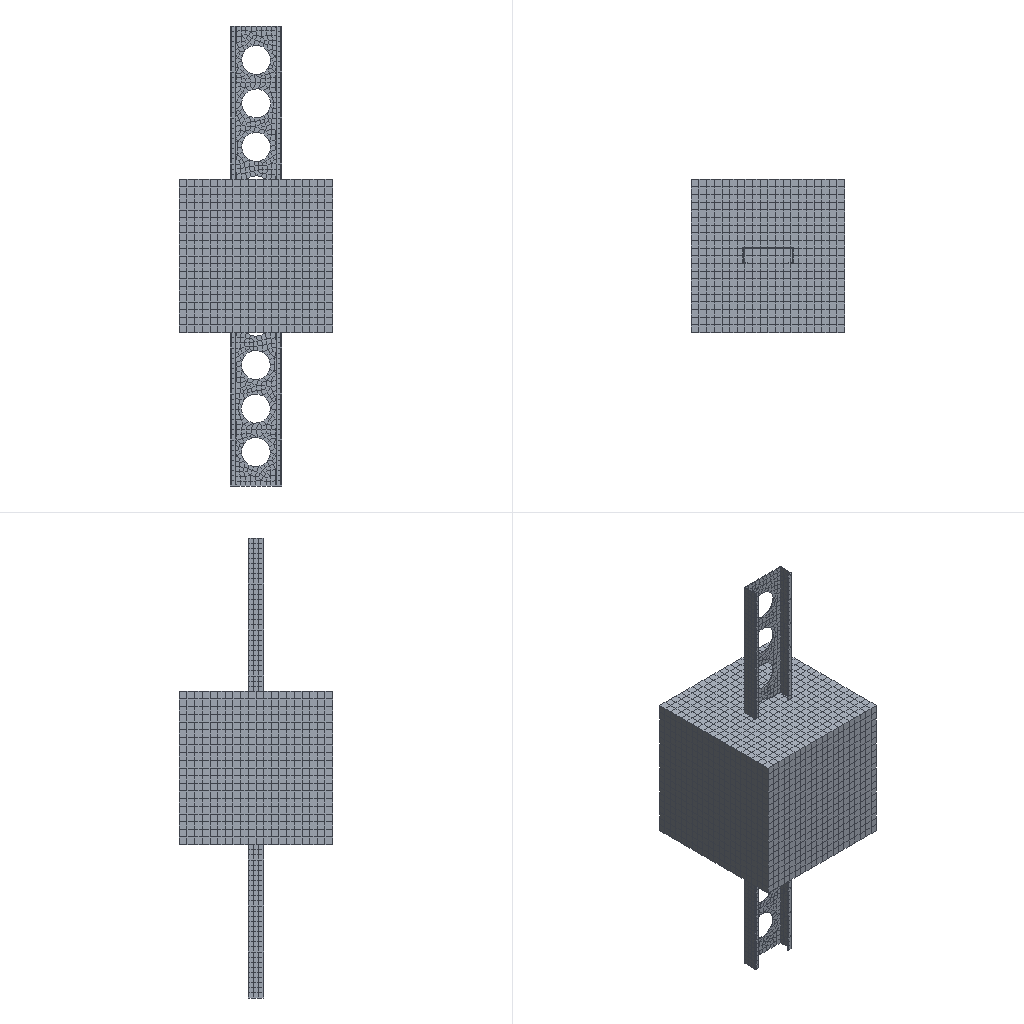Simulation study | abaqus
Set-up summary:
category,name,step,type,value,unit,region
solver,abaqus
solver,version,,,Abaqus/Explicit 2020
units,not stated in the deck,,not stated
analysis,deck,,transient,transient
load_step,Step-1,Step-1,transient
load_step,requested,,,1
mesh,nodes,,,16221
mesh,elements,,,11286
element_type,R3D4,,rigid,192
element_type,C3D8R,,solid,11094
load,load commands in deck,,count,1
bc,support commands in deck,,count,13
material,AL,,in results
material,CON,,in results
material,Q235,,in results
check,setup vs results,,match,"per instance, exact: element labels, types and connectivity; labels of the nodes the elements use; coordinates of those nodes at SINGLE_PRECISION in 7 of 8 instance(s)"
Abaqus input file, long lists of numbers shortened:
*Heading
** Job name: Job-1 Model name: Model-1
** Generated by: Abaqus/CAE 2020
*Preprint, echo=NO, model=NO, history=NO, contact=NO
**
** PARTS
**
*Part, name=Part-1
*Node
      1,        39.75,   29.6,         340.
      2,        39.75,   31.1,         340.
** (2258 more lines like these left out)
*Element, type=C3D8R
 1, 109, 129, 128, 108,   1,   2,   3,   4
 2, 110, 130, 127, 107, 109, 129, 128, 108
** (1014 more lines like these left out)
*Nset, nset=Set-1, generate
    1,  2260,     1
*Elset, elset=Set-1, generate
    1,  1016,     1
** Section: al
*Solid Section, elset=Set-1, material=al
,
*End Part
**
*Part, name=Part-2
*Node
      1,       -27.25,         12.5,         250.
      2,       -27.25,         12.5,           0.
** (2234 more lines like these left out)
*Element, type=C3D8R
 1,   5,  81, 128,   8,   1,  33,  80,   4
 2,  81,  82, 127, 128,  33,  34,  79,  80
** (1060 more lines like these left out)
*Nset, nset=Set-7, generate
    1,  2236,     1
*Elset, elset=Set-7, generate
    1,  1062,     1
** Section: q235
*Solid Section, elset=Set-7, material=q235
,
*End Part
**
*Part, name=Part-3
*Node
      1,          4.5, -0.325,           0.
      2,          4.5,        0.875,           0.
** (48 more lines like these left out)
*Element, type=R3D4
1,  1, 15, 22,  2
2, 15, 14, 21, 22
** (46 more lines like these left out)
*Node
     51,           0.,        0.875,           0.
*Nset, nset=Part-3-RefPt_, internal
51,
*Elset, elset=Part-3, generate
  1,  48,   1
*End Part
**
*Part, name=con
*Node
      1,           0.,        -300.,         300.
      2,           0.,        -285.,         300.
** (9259 more lines like these left out)
*Element, type=C3D8R
   1,  442,  443,  464,  463,    1,    2,   23,   22
   2,  443,  444,  465,  464,    2,    3,   24,   23
** (7998 more lines like these left out)
*Nset, nset=Set-1, generate
    1,  9261,     1
*Elset, elset=Set-1, generate
    1,  8000,     1
** Section: con
*Solid Section, elset=Set-1, material=con
,
*End Part
**
**
** ASSEMBLY
**
*Assembly, name=Assembly
**
*Instance, name=Part-1-1, part=Part-1
*End Instance
**
*Instance, name=Part-1-2, part=Part-1
-17.9,           0.,           0.
-17.9,           0.,           0., -17.9,           1.,           0.,         180.
*End Instance
**
*Instance, name=Part-2-1, part=Part-2
       -31.9,         20.1,        -125.
*End Instance
**
*Instance, name=Part-3-1, part=Part-3
      -34.05,       32.925,        -86.4
*End Instance
**
*Instance, name=Part-3-2, part=Part-3
       16.15,       32.925,        -86.4
*End Instance
**
*Instance, name=Part-3-3, part=Part-3
      -34.05,       32.925,         86.4
*End Instance
**
*Instance, name=Part-3-4, part=Part-3
       16.15,       32.925,         86.4
*End Instance
**
*Instance, name=con-1, part=con
     -158.95,        165.5,        -150.
*End Instance
**
*Node
      1,  -8.95,   15.55,        -450.
*Node
      2,  -8.95,   15.55,         450.
*Nset, nset=Set-5
 1,
*Nset, nset=Set-6
 2,
*Nset, nset=Set-7, instance=Part-3-1
 51,
*Nset, nset=Set-7, instance=Part-3-2
 51,
*Nset, nset=Set-7, instance=Part-3-3
 51,
*Nset, nset=Set-7, instance=Part-3-4
 51,
*Nset, nset=Set-11, instance=Part-2-1
    1,    2,   15,   16,   29,   30,   31,   32,   33,   34,   35,   36,   37,   38,   39,   40
   41,   42,   43,   44,   45,   46,   47,   48,   49,   50,   51,   52,   53,   54,   55,   56
** (55 more lines like these left out)
*Elset, elset=Set-11, instance=Part-2-1, generate
  201,  1062,     1
*Nset, nset=m_Set-1, instance=Part-1-1
   39,   40,   41,   42,   43,   44,   45,   46,   47,   48,   49,   50,   51,   52,   53,   54
   55,   56,   57,   60,   61,   62,   63,   64,   65,   66,   67,   68,   69,   70,   71,   72
** (55 more lines like these left out)
*Nset, nset=m_Set-1, instance=Part-1-2
   39,   40,   41,   42,   43,   44,   45,   46,   47,   48,   49,   50,   51,   52,   53,   54
   55,   56,   57,   60,   61,   62,   63,   64,   65,   66,   67,   68,   69,   70,   71,   72
** (55 more lines like these left out)
*Nset, nset=m_Set-1, instance=Part-3-1, generate
  1,  50,   1
*Nset, nset=m_Set-1, instance=Part-3-3, generate
  1,  50,   1
*Nset, nset=m_Set-1, instance=Part-3-2, generate
  1,  50,   1
*Nset, nset=m_Set-1, instance=Part-3-4, generate
  1,  50,   1
*Elset, elset=m_Set-1, instance=Part-1-1
  361,  362,  363,  364,  365,  366,  367,  368,  369,  370,  371,  372,  373,  374,  375,  376
  377,  378,  379,  380,  381,  382,  383,  384,  385,  386,  387,  388,  389,  390,  391,  392
** (23 more lines like these left out)
*Elset, elset=m_Set-1, instance=Part-1-2
  361,  362,  363,  364,  365,  366,  367,  368,  369,  370,  371,  372,  373,  374,  375,  376
  377,  378,  379,  380,  381,  382,  383,  384,  385,  386,  387,  388,  389,  390,  391,  392
** (23 more lines like these left out)
*Elset, elset=m_Set-1, instance=Part-3-1, generate
  1,  48,   1
*Elset, elset=m_Set-1, instance=Part-3-3, generate
  1,  48,   1
*Elset, elset=m_Set-1, instance=Part-3-2, generate
  1,  48,   1
*Elset, elset=m_Set-1, instance=Part-3-4, generate
  1,  48,   1
*Nset, nset=m_Set-3
 1,
*Nset, nset=m_Set-4
 2,
*Nset, nset=m_Set-9, instance=Part-1-1
   39,   40,   41,   42,   43,   44,   45,   46,   47,   48,   49,   50,   51,   52,   53,   54
   55,   56,   57,   60,   61,   62,   63,   64,   65,   66,   67,   68,   69,   70,   71,   72
** (55 more lines like these left out)
*Nset, nset=m_Set-9, instance=Part-1-2
   39,   40,   41,   42,   43,   44,   45,   46,   47,   48,   49,   50,   51,   52,   53,   54
   55,   56,   57,   60,   61,   62,   63,   64,   65,   66,   67,   68,   69,   70,   71,   72
** (55 more lines like these left out)
*Nset, nset=m_Set-9, instance=Part-3-1, generate
  1,  50,   1
*Nset, nset=m_Set-9, instance=Part-3-3, generate
  1,  50,   1
*Nset, nset=m_Set-9, instance=Part-2-1, generate
    1,  2236,     1
*Nset, nset=m_Set-9, instance=Part-3-2, generate
  1,  50,   1
*Nset, nset=m_Set-9, instance=Part-3-4, generate
  1,  50,   1
*Elset, elset=m_Set-9, instance=Part-1-1
  361,  362,  363,  364,  365,  366,  367,  368,  369,  370,  371,  372,  373,  374,  375,  376
  377,  378,  379,  380,  381,  382,  383,  384,  385,  386,  387,  388,  389,  390,  391,  392
** (23 more lines like these left out)
*Elset, elset=m_Set-9, instance=Part-1-2
  361,  362,  363,  364,  365,  366,  367,  368,  369,  370,  371,  372,  373,  374,  375,  376
  377,  378,  379,  380,  381,  382,  383,  384,  385,  386,  387,  388,  389,  390,  391,  392
** (23 more lines like these left out)
*Elset, elset=m_Set-9, instance=Part-3-1, generate
  1,  48,   1
*Elset, elset=m_Set-9, instance=Part-3-3, generate
  1,  48,   1
*Elset, elset=m_Set-9, instance=Part-2-1, generate
    1,  1062,     1
*Elset, elset=m_Set-9, instance=Part-3-2, generate
  1,  48,   1
*Elset, elset=m_Set-9, instance=Part-3-4, generate
  1,  48,   1
*Nset, nset=s_Set-1, instance=con-1, generate
    1,  9261,     1
*Elset, elset=s_Set-1, instance=con-1, generate
    1,  8000,     1
*Nset, nset=s_Set-9, instance=con-1, generate
    1,  9261,     1
*Elset, elset=s_Set-9, instance=con-1, generate
    1,  8000,     1
*Elset, elset=_m_Surf-3_S5, internal, instance=Part-1-1
  361,  362,  363,  364,  365,  366,  367,  368,  369,  370,  371,  372,  373,  374,  375,  376
  377,  378,  379,  380,  381,  382,  383,  384,  385,  386,  387,  388,  389,  390,  436,  437
** (3 more lines like these left out)
*Elset, elset=_m_Surf-3_S4, internal, instance=Part-1-1
  361,  362,  363,  364,  365,  366,  367,  368,  369,  370,  371,  372,  373,  374,  375,  376
  377,  378,  379,  380,  381,  382,  383,  384,  385,  386,  387,  388,  389,  390,  391,  392
** (9 more lines like these left out)
*Elset, elset=_m_Surf-3_S3, internal, instance=Part-1-1
 466, 467, 468, 469, 470, 471, 472, 473, 474, 475, 476, 477, 478, 479, 480, 814
 851, 878, 920, 981
*Elset, elset=_m_Surf-3_S2, internal, instance=Part-1-1, generate
  802,  1016,     1
*Elset, elset=_m_Surf-3_S6, internal, instance=Part-1-1
 376, 377, 378, 379, 380, 381, 382, 383, 384, 385, 386, 387, 388, 389, 390, 391
 392, 393, 394, 395, 396, 397, 398, 399, 400, 401, 402, 403, 404, 405, 406, 407
** (7 more lines like these left out)
*Elset, elset=_m_Surf-3_S1, internal, instance=Part-1-1, generate
  802,  1016,     1
*Surface, type=ELEMENT, name=m_Surf-3
_m_Surf-3_S5, S5
_m_Surf-3_S4, S4
_m_Surf-3_S2, S2
_m_Surf-3_S6, S6
_m_Surf-3_S3, S3
_m_Surf-3_S1, S1
*Elset, elset=_m_Surf-6_SPOS, internal, instance=Part-3-4, generate
  1,  48,   1
*Surface, type=ELEMENT, name=m_Surf-6
_m_Surf-6_SPOS, SPOS
*Elset, elset=_m_Surf-8_SPOS, internal, instance=Part-3-3, generate
  1,  48,   1
*Surface, type=ELEMENT, name=m_Surf-8
_m_Surf-8_SPOS, SPOS
*Elset, elset=_m_Surf-10_S5, internal, instance=Part-1-2
  361,  362,  363,  364,  365,  366,  367,  368,  369,  370,  371,  372,  373,  374,  375,  376
  377,  378,  379,  380,  381,  382,  383,  384,  385,  386,  387,  388,  389,  390,  436,  437
** (3 more lines like these left out)
*Elset, elset=_m_Surf-10_S4, internal, instance=Part-1-2
  361,  362,  363,  364,  365,  366,  367,  368,  369,  370,  371,  372,  373,  374,  375,  376
  377,  378,  379,  380,  381,  382,  383,  384,  385,  386,  387,  388,  389,  390,  391,  392
** (9 more lines like these left out)
*Elset, elset=_m_Surf-10_S3, internal, instance=Part-1-2
 466, 467, 468, 469, 470, 471, 472, 473, 474, 475, 476, 477, 478, 479, 480, 814
 851, 878, 920, 981
*Elset, elset=_m_Surf-10_S2, internal, instance=Part-1-2, generate
  802,  1016,     1
*Elset, elset=_m_Surf-10_S6, internal, instance=Part-1-2
 376, 377, 378, 379, 380, 381, 382, 383, 384, 385, 386, 387, 388, 389, 390, 391
 392, 393, 394, 395, 396, 397, 398, 399, 400, 401, 402, 403, 404, 405, 406, 407
** (7 more lines like these left out)
*Elset, elset=_m_Surf-10_S1, internal, instance=Part-1-2, generate
  802,  1016,     1
*Surface, type=ELEMENT, name=m_Surf-10
_m_Surf-10_S5, S5
_m_Surf-10_S4, S4
_m_Surf-10_S2, S2
_m_Surf-10_S6, S6
_m_Surf-10_S3, S3
_m_Surf-10_S1, S1
*Elset, elset=_m_Surf-13_SPOS, internal, instance=Part-3-1, generate
  1,  48,   1
*Surface, type=ELEMENT, name=m_Surf-13
_m_Surf-13_SPOS, SPOS
*Elset, elset=_m_Surf-15_SPOS, internal, instance=Part-3-2, generate
  1,  48,   1
*Surface, type=ELEMENT, name=m_Surf-15
_m_Surf-15_SPOS, SPOS
*Elset, elset=_m_Surf-16_SPOS, internal, instance=Part-3-4, generate
  1,  48,   1
*Surface, type=ELEMENT, name=m_Surf-16
_m_Surf-16_SPOS, SPOS
*Elset, elset=_m_Surf-17_SPOS, internal, instance=Part-3-3, generate
  1,  48,   1
*Surface, type=ELEMENT, name=m_Surf-17
_m_Surf-17_SPOS, SPOS
*Elset, elset=_s_Surf-1_S4, internal, instance=Part-1-2
   1,   2,   3,   4,   5,   6,   7,   8,   9,  10,  11,  12,  13,  14,  15,  16
  17,  18,  19,  20,  21,  22,  23,  24,  25,  26,  27,  28,  29,  30,  31,  32
** (7 more lines like these left out)
*Elset, elset=_s_Surf-1_S5, internal, instance=Part-1-2
   1,   2,   3,   4,   5,   6,   7,   8,   9,  10,  11,  12,  13,  14,  15,  16
  17,  18,  19,  20,  21,  22,  56,  57,  58,  59,  60,  61,  62,  63,  64,  65
** (1 more lines like these left out)
*Elset, elset=_s_Surf-1_S2, internal, instance=Part-1-2
 331, 332, 333, 334, 335, 336, 337, 338, 339, 340, 341, 541, 542, 543, 544, 545
 546, 547, 548, 549, 550, 551, 552, 553, 554, 555, 556, 557, 558, 559, 560, 561
** (5 more lines like these left out)
*Elset, elset=_s_Surf-1_S3, internal, instance=Part-1-2
 111, 112, 113, 114, 115, 116, 117, 118, 119, 120, 121, 551, 574, 585, 597
*Elset, elset=_s_Surf-1_S6, internal, instance=Part-1-2
  12,  13,  14,  15,  16,  17,  18,  19,  20,  21,  22,  23,  24,  25,  26,  27
  28,  29,  30,  31,  32,  33,  34,  35,  36,  37,  38,  39,  40,  41,  42,  43
** (5 more lines like these left out)
*Elset, elset=_s_Surf-1_S1, internal, instance=Part-1-2
  11,  22,  53,  54,  55,  66,  77, 108, 109, 110, 121, 541, 542, 543, 544, 545
 546, 547, 548, 549, 550, 551, 552, 553, 554, 555, 556, 557, 558, 559, 560, 561
** (5 more lines like these left out)
*Surface, type=ELEMENT, name=s_Surf-1
_s_Surf-1_S4, S4
_s_Surf-1_S5, S5
_s_Surf-1_S2, S2
_s_Surf-1_S6, S6
_s_Surf-1_S3, S3
_s_Surf-1_S1, S1
*Elset, elset=_s_Surf-2_S4, internal, instance=Part-1-1
   1,   2,   3,   4,   5,   6,   7,   8,   9,  10,  11,  12,  13,  14,  15,  16
  17,  18,  19,  20,  21,  22,  23,  24,  25,  26,  27,  28,  29,  30,  31,  32
** (7 more lines like these left out)
*Elset, elset=_s_Surf-2_S5, internal, instance=Part-1-1
   1,   2,   3,   4,   5,   6,   7,   8,   9,  10,  11,  12,  13,  14,  15,  16
  17,  18,  19,  20,  21,  22,  56,  57,  58,  59,  60,  61,  62,  63,  64,  65
** (1 more lines like these left out)
*Elset, elset=_s_Surf-2_S2, internal, instance=Part-1-1
 331, 332, 333, 334, 335, 336, 337, 338, 339, 340, 341, 541, 542, 543, 544, 545
 546, 547, 548, 549, 550, 551, 552, 553, 554, 555, 556, 557, 558, 559, 560, 561
** (5 more lines like these left out)
*Elset, elset=_s_Surf-2_S3, internal, instance=Part-1-1
 111, 112, 113, 114, 115, 116, 117, 118, 119, 120, 121, 551, 574, 585, 597
*Elset, elset=_s_Surf-2_S6, internal, instance=Part-1-1
  12,  13,  14,  15,  16,  17,  18,  19,  20,  21,  22,  23,  24,  25,  26,  27
  28,  29,  30,  31,  32,  33,  34,  35,  36,  37,  38,  39,  40,  41,  42,  43
** (5 more lines like these left out)
*Elset, elset=_s_Surf-2_S1, internal, instance=Part-1-1
  11,  22,  53,  54,  55,  66,  77, 108, 109, 110, 121, 541, 542, 543, 544, 545
 546, 547, 548, 549, 550, 551, 552, 553, 554, 555, 556, 557, 558, 559, 560, 561
** (5 more lines like these left out)
*Surface, type=ELEMENT, name=s_Surf-2
_s_Surf-2_S4, S4
_s_Surf-2_S5, S5
_s_Surf-2_S2, S2
_s_Surf-2_S6, S6
_s_Surf-2_S3, S3
_s_Surf-2_S1, S1
*Elset, elset=_s_Surf-3_S6, internal, instance=Part-2-1
  1, 26
*Elset, elset=_s_Surf-3_S3, internal, instance=Part-2-1
  51,  52,  53, 126, 151, 176
*Surface, type=ELEMENT, name=s_Surf-3
_s_Surf-3_S6, S6
_s_Surf-3_S3, S3
*Elset, elset=_s_Surf-6_S6, internal, instance=Part-1-1
 805, 900
*Elset, elset=_s_Surf-6_S3, internal, instance=Part-1-1
 810, 812, 813
*Elset, elset=_s_Surf-6_S4, internal, instance=Part-1-1
 869, 881, 882
*Surface, type=ELEMENT, name=s_Surf-6
_s_Surf-6_S6, S6
_s_Surf-6_S3, S3
_s_Surf-6_S4, S4
*Elset, elset=_s_Surf-8_S4, internal, instance=Part-1-1
 821, 879, 887
*Elset, elset=_s_Surf-8_S3, internal, instance=Part-1-1
 822,
*Elset, elset=_s_Surf-8_S6, internal, instance=Part-1-1
 835, 885
*Elset, elset=_s_Surf-8_S5, internal, instance=Part-1-1
 883, 886
*Surface, type=ELEMENT, name=s_Surf-8
_s_Surf-8_S4, S4
_s_Surf-8_S3, S3
_s_Surf-8_S6, S6
_s_Surf-8_S5, S5
*Elset, elset=_s_Surf-12_S1, internal, instance=Part-2-1, generate
  201,  1062,     1
*Elset, elset=_s_Surf-12_S4, internal, instance=Part-2-1, generate
 126,  200,    1
*Elset, elset=_s_Surf-12_S2, internal, instance=Part-2-1, generate
  51,  125,    1
*Surface, type=ELEMENT, name=s_Surf-12
_s_Surf-12_S1, S1
_s_Surf-12_S4, S4
_s_Surf-12_S2, S2
*Elset, elset=_s_Surf-13_S2, internal, instance=Part-2-1, generate
  201,  1062,     1
*Surface, type=ELEMENT, name=s_Surf-13
_s_Surf-13_S2, S2
*Rigid Body, ref node=Part-3-1.Part-3-RefPt_, elset=Part-3-1.Part-3
*Rigid Body, ref node=Part-3-2.Part-3-RefPt_, elset=Part-3-2.Part-3
*Rigid Body, ref node=Part-3-3.Part-3-RefPt_, elset=Part-3-3.Part-3
*Rigid Body, ref node=Part-3-4.Part-3-RefPt_, elset=Part-3-4.Part-3
** Constraint: Constraint-2
*Coupling, constraint name=Constraint-2, ref node=m_Set-3, surface=s_Surf-1
*Kinematic
** Constraint: Constraint-3
*Coupling, constraint name=Constraint-3, ref node=m_Set-4, surface=s_Surf-2
*Kinematic
** Constraint: Constraint-4
*Embedded Element, host elset=s_Set-9
m_Set-9
*End Assembly
**
** MATERIALS
**
*Material, name=al
*Damage Initiation, criterion=SHEAR
 0.1,0.,0.
*Damage Evolution, type=DISPLACEMENT
 0.006,
*Density
 2.7e-09,
*Elastic
72000., 0.33
*Plastic
400.,0.
*Material, name=con
*Density
 2.2e-09,
*Elastic
29791., 0.2
*Concrete Damaged Plasticity
30.,    0.1,   1.16, 0.6667,   0.05
*Concrete Compression Hardening
 15.4,      0.
 16.9,  0.0002
 19.6, 0.00048
 20.1, 0.00079
  20., 0.00095
 19.6,  0.0011
 19.1, 0.00127
 18.6, 0.00143
 17.9,  0.0016
 17.2, 0.00177
 16.6, 0.00194
 15.9, 0.00211
 15.3, 0.00228
 14.7, 0.00245
 14.1, 0.00261
 13.5, 0.00278
  13., 0.00294
 12.5,  0.0031
  12., 0.00327
 11.6, 0.00343
 11.2, 0.00359
 10.8, 0.00375
 10.4, 0.00391
 10.1, 0.00406
*Concrete Tension Stiffening
 2.06,      0.
 1.92,   2e-05
 1.72,   4e-05
 1.53,   6e-05
 1.37,   8e-05
 1.24,  0.0001
 1.13, 0.00011
 1.04, 0.00013
 0.97, 0.00015
  0.9, 0.00016
 0.85, 0.00018
*Concrete Compression Damage
     0.,      0.
 0.0841,   9e-05
 0.0933,  0.0001
 0.1091, 0.00013
 0.1418,  0.0002
 0.2407, 0.00048
  0.322, 0.00079
 0.3557, 0.00095
 0.3886,  0.0011
 0.4201, 0.00127
 0.4499, 0.00143
 0.4778,  0.0016
 0.5039, 0.00177
 0.5282, 0.00194
 0.5506, 0.00211
 0.5715, 0.00228
 0.5908, 0.00245
 0.6086, 0.00261
 0.6252, 0.00278
 0.6406, 0.00294
 0.6549,  0.0031
 0.6682, 0.00327
 0.6806, 0.00343
 0.6922, 0.00359
  0.703, 0.00375
 0.7131, 0.00391
 0.7227, 0.00406
   0.74, 0.00438
 0.7554, 0.00469
 0.7691,   0.005
 0.7815, 0.00531
 0.7926, 0.00561
 0.8026, 0.00592
 0.8118, 0.00622
 0.8202, 0.00653
 0.8278, 0.00683
 0.8349, 0.00713
*Concrete Tension Damage
      0.,      0.
 0.1181,   2e-05
 0.2281,   4e-05
 0.3187,   6e-05
 0.3919,   8e-05
 0.4512,  0.0001
 0.5, 0.00011
  0.5407, 0.00013
 0.575, 0.00015
 0.6043, 0.00016
 0.6297, 0.00018
 0.7177, 0.00025
 0.7702, 0.00033
 0.8053,  0.0004
 0.8304, 0.00047
 0.8494, 0.00054
  0.8643, 0.00061
 0.8763, 0.00068
 0.8862, 0.00075
*CONCRETE FAILURE
0.0001,0,0,0
*Material, name=q235
*Density
 7.8e-09,
*Elastic
210000., 0.3
*Plastic
235.,0.
**
** INTERACTION PROPERTIES
**
*Surface Interaction, name=IntProp-1
*Friction
 0.2,
*Surface Behavior, pressure-overclosure=HARD
** ----------------------------------------------------------------
**
** STEP: Step-1
**
*Step, name=Step-1, nlgeom=YES
*Dynamic, Explicit
, 0.08
*Bulk Viscosity
0.06, 1.2
** Mass Scaling: Semi-Automatic
**               Whole Model
*Fixed Mass Scaling, factor=50.
**
** BOUNDARY CONDITIONS
**
** Name: BC-1 Type: 对称/反对称/完全固定
*Boundary
Set-5, ENCASTRE
** Name: [REDACTED] : Displacement/rotation angle
*Boundary
Set-7, 1, 1
Set-7, 2, 2
Set-7, 3, 3
Set-7, 4, 4
Set-7, 5, 5
Set-7, 6, 6
** Name: [REDACTED] : Velocity/Angular velocity
*Boundary, type=VELOCITY
Set-6, 1, 1
Set-6, 2, 2
Set-6, 3, 3, 100.
Set-6, 4, 4
Set-6, 5, 5
Set-6, 6, 6
**
** INTERACTIONS
**
** Interaction: Int-2
*Contact Pair, interaction=IntProp-1, mechanical constraint=KINEMATIC, cpset=Int-2
s_Surf-12, m_Surf-3
** Interaction: Int-3
*Contact Pair, interaction=IntProp-1, mechanical constraint=PENALTY, cpset=Int-3
m_Surf-6, s_Surf-6
** Interaction: Int-4
*Contact Pair, interaction=IntProp-1, mechanical constraint=PENALTY, cpset=Int-4
m_Surf-8, s_Surf-8
** Interaction: Int-5
*Contact Pair, interaction=IntProp-1, mechanical constraint=KINEMATIC, cpset=Int-5
m_Surf-10, s_Surf-12
** Interaction: Int-1
*Contact, op=NEW
*Contact Inclusions, ALL EXTERIOR
*Contact Property Assignment
 ,  , IntProp-1
**
** OUTPUT REQUESTS
**
*Restart, write, number interval=1, time marks=NO
**
** FIELD OUTPUT: F-Output-1
**
*Output, field, number interval=50
*Node Output
A, CF, RF, RM, RT, U, V
*Element Output, directions=YES
DAMAGEC, DAMAGET, E, EVF, LE, MISES, PE, PEEQ, PEEQVAVG, PEVAVG, S, SDEG, STATUS, SVAVG
*Contact Output
CDISP, CSTRESS
**
** HISTORY OUTPUT: H-Output-1
**
*Output, history, variable=PRESELECT
*End Step
Results summary:
result,step,Step-1,partial,increments=51278 time=0.07311/0.08
result,analysis,,,transient
result,last_loadstep,,,1
result,primary field,,,U
result,reaction total,,FX,0.0,model units
result,reaction total,,FY,0.0,model units
result,reaction total,,FZ,0.0,model units